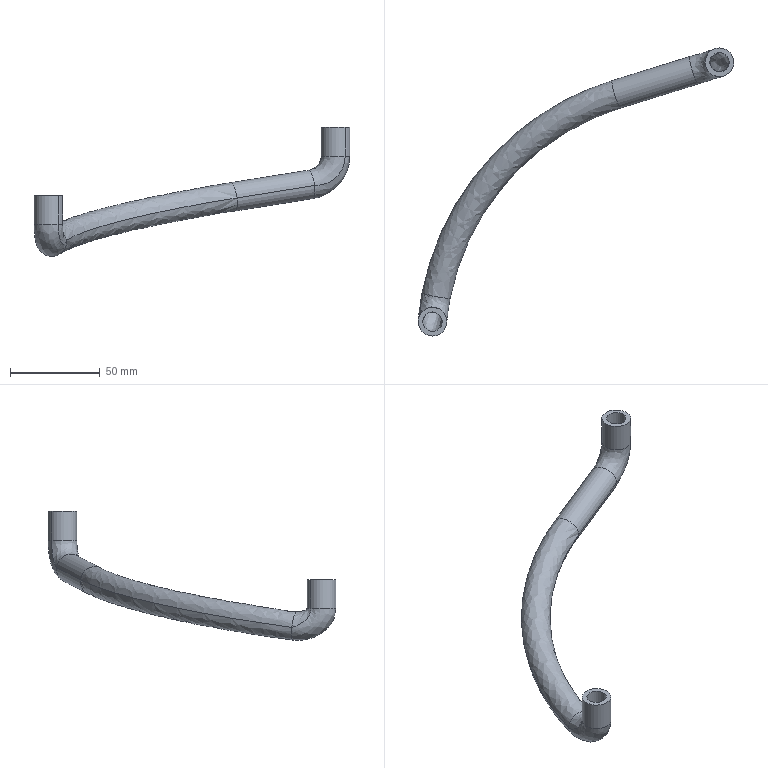Part | STEP file | GUANLU-XIAOPENBI | 1 solid | 26 faces | box 176 x 160.5 x 71.93 mm | volume 30798 mm3 | cylinder 12 | spline 12 | plane 2 | commonest cylinder face diameters 10.8 x6 16 x6